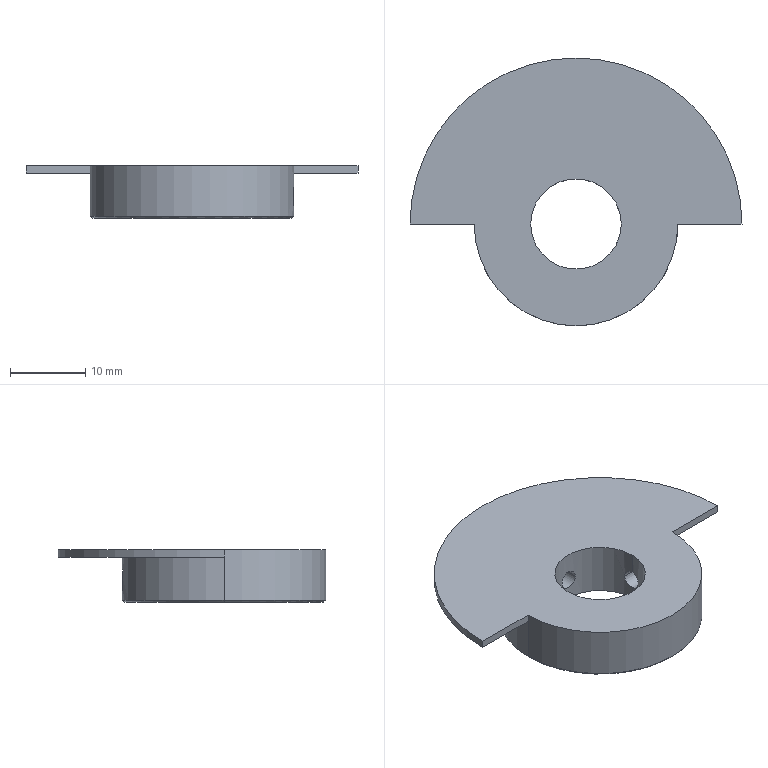Part | NX | 1 solid | 20 faces | box 44 x 35.5 x 7 mm | volume 3612 mm3 | cylinder 9 | plane 5 | spline 4 | cone 2 | commonest cylinder face diameters 2.5 x4 12 x2 27 x2 44 x1
STEP:
#1=CARTESIAN_POINT('',(-13.2,0.,-7.));
#2=VERTEX_POINT('',#1);
#3=CARTESIAN_POINT('',(13.2,0.,-7.));
#4=VERTEX_POINT('',#3);
#5=CARTESIAN_POINT('',(0.,0.,-7.));
#6=DIRECTION('',(0.,0.,-1.));
#7=DIRECTION('',(1.,0.,0.));
#8=AXIS2_PLACEMENT_3D('',#5,#6,#7);
#9=CIRCLE('',#8,13.2);
#10=EDGE_CURVE('',#2,#4,#9,.T.);
#11=ORIENTED_EDGE('',*,*,#10,.T.);
#12=CARTESIAN_POINT('',(0.,0.,-7.));
#13=DIRECTION('',(0.,0.,-1.));
#14=DIRECTION('',(1.,0.,0.));
#15=AXIS2_PLACEMENT_3D('',#12,#13,#14);
#16=CIRCLE('',#15,13.2);
#17=EDGE_CURVE('',#4,#2,#16,.T.);
#18=ORIENTED_EDGE('',*,*,#17,.T.);
#19=EDGE_LOOP('',(#11,#18));
#20=FACE_BOUND('',#19,.T.);
#21=CARTESIAN_POINT('',(-6.,0.,-7.));
#22=VERTEX_POINT('',#21);
#23=CARTESIAN_POINT('',(6.,0.,-7.));
#24=VERTEX_POINT('',#23);
#25=CARTESIAN_POINT('',(0.,0.,-7.));
#26=DIRECTION('',(0.,0.,1.));
#27=DIRECTION('',(1.,0.,0.));
#28=AXIS2_PLACEMENT_3D('',#25,#26,#27);
#29=CIRCLE('',#28,6.);
#30=EDGE_CURVE('',#22,#24,#29,.T.);
#31=ORIENTED_EDGE('',*,*,#30,.T.);
#32=CARTESIAN_POINT('',(0.,0.,-7.));
#33=DIRECTION('',(0.,0.,1.));
#34=DIRECTION('',(1.,0.,0.));
#35=AXIS2_PLACEMENT_3D('',#32,#33,#34);
#36=CIRCLE('',#35,6.);
#37=EDGE_CURVE('',#24,#22,#36,.T.);
#38=ORIENTED_EDGE('',*,*,#37,.T.);
#39=EDGE_LOOP('',(#31,#38));
#40=FACE_BOUND('',#39,.T.);
#41=CARTESIAN_POINT('',(0.,0.,-7.));
#42=DIRECTION('',(0.,0.,1.));
#43=DIRECTION('',(1.,0.,0.));
#44=AXIS2_PLACEMENT_3D('',#41,#42,#43);
#45=PLANE('',#44);
#46=ADVANCED_FACE('',(#20,#40),#45,.F.);
#47=CARTESIAN_POINT('',(-13.5,0.,0.));
#48=VERTEX_POINT('',#47);
#49=CARTESIAN_POINT('',(13.5,0.,0.));
#50=VERTEX_POINT('',#49);
#51=CARTESIAN_POINT('',(0.,0.,0.));
#52=DIRECTION('',(0.,0.,1.));
#53=DIRECTION('',(-1.,0.,0.));
#54=AXIS2_PLACEMENT_3D('',#51,#52,#53);
#55=CIRCLE('',#54,13.5);
#56=EDGE_CURVE('',#48,#50,#55,.T.);
#57=ORIENTED_EDGE('',*,*,#56,.F.);
#58=CARTESIAN_POINT('',(-13.5,0.,-1.));
#59=VERTEX_POINT('',#58);
#60=CARTESIAN_POINT('',(-13.5,0.,0.));
#61=DIRECTION('',(0.,0.,-1.));
#62=VECTOR('',#61,1000.);
#63=LINE('',#60,#62);
#64=EDGE_CURVE('',#48,#59,#63,.T.);
#65=ORIENTED_EDGE('',*,*,#64,.T.);
#66=CARTESIAN_POINT('',(-13.5,0.,-6.7));
#67=VERTEX_POINT('',#66);
#68=CARTESIAN_POINT('',(-13.5,0.,0.));
#69=DIRECTION('',(0.,0.,-1.));
#70=VECTOR('',#69,1000.);
#71=LINE('',#68,#70);
#72=EDGE_CURVE('',#67,#59,#71,.F.);
#73=ORIENTED_EDGE('',*,*,#72,.F.);
#74=CARTESIAN_POINT('',(13.5,0.,-6.7));
#75=VERTEX_POINT('',#74);
#76=CARTESIAN_POINT('',(0.,0.,-6.7));
#77=DIRECTION('',(0.,0.,-1.));
#78=DIRECTION('',(1.,0.,0.));
#79=AXIS2_PLACEMENT_3D('',#76,#77,#78);
#80=CIRCLE('',#79,13.5);
#81=EDGE_CURVE('',#75,#67,#80,.T.);
#82=ORIENTED_EDGE('',*,*,#81,.F.);
#83=CARTESIAN_POINT('',(13.5,0.,-5.7));
#84=VERTEX_POINT('',#83);
#85=CARTESIAN_POINT('',(13.5,0.,0.));
#86=DIRECTION('',(0.,0.,-1.));
#87=VECTOR('',#86,1000.);
#88=LINE('',#85,#87);
#89=EDGE_CURVE('',#84,#75,#88,.T.);
#90=ORIENTED_EDGE('',*,*,#89,.F.);
#91=CARTESIAN_POINT('',(13.5,-0.01096,-5.7));
#92=VERTEX_POINT('',#91);
#93=CARTESIAN_POINT('',(13.5,0.,-5.7));
#94=CARTESIAN_POINT('',(13.5,-0.003653,-5.7));
#95=CARTESIAN_POINT('',(13.5,-0.007306,-5.7));
#96=CARTESIAN_POINT('',(13.5,-0.01096,-5.7));
#97=B_SPLINE_CURVE_WITH_KNOTS('',3,(#93,#94,#95,#96),.UNSPECIFIED.,.F.,.F.,(4,4),(0.,1.),.UNSPECIFIED.);
#98=EDGE_CURVE('',#84,#92,#97,.T.);
#99=ORIENTED_EDGE('',*,*,#98,.T.);
#100=CARTESIAN_POINT('',(13.5,0.,-2.3));
#101=VERTEX_POINT('',#100);
#102=CARTESIAN_POINT('',(13.5,-0.01096,-5.7));
#103=CARTESIAN_POINT('',(13.499,-0.9006,-5.694));
#104=CARTESIAN_POINT('',(13.303,-2.364,-3.994));
#105=CARTESIAN_POINT('',(13.5,-0.8891,-2.3));
#106=CARTESIAN_POINT('',(13.5,0.,-2.3));
#107=B_SPLINE_CURVE_WITH_KNOTS('',3,(#102,#103,#104,#105,#106),.UNSPECIFIED.,.F.,.F.,(4,1,4),(0.,0.5,1.),.UNSPECIFIED.);
#108=EDGE_CURVE('',#92,#101,#107,.T.);
#109=ORIENTED_EDGE('',*,*,#108,.T.);
#110=CARTESIAN_POINT('',(13.5,0.,-1.));
#111=VERTEX_POINT('',#110);
#112=CARTESIAN_POINT('',(13.5,0.,0.));
#113=DIRECTION('',(0.,0.,-1.));
#114=VECTOR('',#113,1000.);
#115=LINE('',#112,#114);
#116=EDGE_CURVE('',#101,#111,#115,.F.);
#117=ORIENTED_EDGE('',*,*,#116,.T.);
#118=CARTESIAN_POINT('',(13.5,0.,0.));
#119=DIRECTION('',(0.,0.,-1.));
#120=VECTOR('',#119,1000.);
#121=LINE('',#118,#120);
#122=EDGE_CURVE('',#50,#111,#121,.T.);
#123=ORIENTED_EDGE('',*,*,#122,.F.);
#124=EDGE_LOOP('',(#57,#65,#73,#82,#90,#99,#109,#117,#123));
#125=FACE_BOUND('',#124,.T.);
#126=CARTESIAN_POINT('',(0.,0.,0.));
#127=DIRECTION('',(0.,0.,-1.));
#128=DIRECTION('',(-1.,0.,0.));
#129=AXIS2_PLACEMENT_3D('',#126,#127,#128);
#130=CYLINDRICAL_SURFACE('',#129,13.5);
#131=ADVANCED_FACE('',(#125),#130,.T.);
#132=CARTESIAN_POINT('',(0.009525,13.24,-5.25));
#133=VERTEX_POINT('',#132);
#134=CARTESIAN_POINT('',(1.25,13.182,-4.));
#135=VERTEX_POINT('',#134);
#136=CARTESIAN_POINT('',(1.25,13.182,-4.));
#137=CARTESIAN_POINT('',(1.25,13.182,-4.158));
#138=CARTESIAN_POINT('',(1.181,13.188,-4.446));
#139=CARTESIAN_POINT('',(1.074,13.198,-4.653));
#140=CARTESIAN_POINT('',(0.8909,13.211,-4.899));
#141=CARTESIAN_POINT('',(0.6426,13.225,-5.08));
#142=CARTESIAN_POINT('',(0.4451,13.234,-5.18));
#143=CARTESIAN_POINT('',(0.1615,13.24,-5.249));
#144=CARTESIAN_POINT('',(0.009525,13.24,-5.25));
#145=B_SPLINE_CURVE_WITH_KNOTS('',3,(#136,#137,#138,#139,#140,#141,#142,#143,#144),.UNSPECIFIED.,.F.,.F.,(4,1,1,1,1,1,4),(0.,0.25,0.375,0.5,0.625,0.75,1.),.UNSPECIFIED.);
#146=EDGE_CURVE('',#133,#135,#145,.F.);
#147=ORIENTED_EDGE('',*,*,#146,.T.);
#148=CARTESIAN_POINT('',(-0.009148,13.24,-2.75));
#149=VERTEX_POINT('',#148);
#150=CARTESIAN_POINT('',(-0.009147,13.24,-2.75));
#151=CARTESIAN_POINT('',(0.1457,13.24,-2.749));
#152=CARTESIAN_POINT('',(0.4278,13.234,-2.813));
#153=CARTESIAN_POINT('',(0.6331,13.225,-2.915));
#154=CARTESIAN_POINT('',(0.8826,13.212,-3.093));
#155=CARTESIAN_POINT('',(1.072,13.198,-3.344));
#156=CARTESIAN_POINT('',(1.178,13.189,-3.548));
#157=CARTESIAN_POINT('',(1.25,13.182,-3.841));
#158=CARTESIAN_POINT('',(1.25,13.182,-4.));
#159=B_SPLINE_CURVE_WITH_KNOTS('',3,(#150,#151,#152,#153,#154,#155,#156,#157,#158),.UNSPECIFIED.,.F.,.F.,(4,1,1,1,1,1,4),(0.,0.25,0.375,0.5,0.625,0.75,1.),.UNSPECIFIED.);
#160=EDGE_CURVE('',#135,#149,#159,.F.);
#161=ORIENTED_EDGE('',*,*,#160,.T.);
#162=CARTESIAN_POINT('',(-0.01305,13.5,-2.3));
#163=VERTEX_POINT('',#162);
#164=CARTESIAN_POINT('',(-0.009148,13.24,-2.75));
#165=CARTESIAN_POINT('',(-0.01305,13.5,-2.3));
#166=B_SPLINE_CURVE_WITH_KNOTS('',1,(#164,#165),.UNSPECIFIED.,.F.,.F.,(2,2),(0.,1.),.UNSPECIFIED.);
#167=EDGE_CURVE('',#163,#149,#166,.F.);
#168=ORIENTED_EDGE('',*,*,#167,.F.);
#169=CARTESIAN_POINT('',(0.01314,13.5,-5.7));
#170=VERTEX_POINT('',#169);
#171=CARTESIAN_POINT('',(0.01314,13.5,-5.7));
#172=CARTESIAN_POINT('',(0.9097,13.499,-5.692));
#173=CARTESIAN_POINT('',(2.362,13.303,-3.98));
#174=CARTESIAN_POINT('',(0.8851,13.501,-2.294));
#175=CARTESIAN_POINT('',(-0.01305,13.5,-2.3));
#176=B_SPLINE_CURVE_WITH_KNOTS('',3,(#171,#172,#173,#174,#175),.UNSPECIFIED.,.F.,.F.,(4,1,4),(0.,0.5,1.),.UNSPECIFIED.);
#177=EDGE_CURVE('',#170,#163,#176,.T.);
#178=ORIENTED_EDGE('',*,*,#177,.F.);
#179=CARTESIAN_POINT('',(0.009525,13.24,-5.25));
#180=CARTESIAN_POINT('',(0.01314,13.5,-5.7));
#181=B_SPLINE_CURVE_WITH_KNOTS('',1,(#179,#180),.UNSPECIFIED.,.F.,.F.,(2,2),(0.,1.),.UNSPECIFIED.);
#182=EDGE_CURVE('',#170,#133,#181,.F.);
#183=ORIENTED_EDGE('',*,*,#182,.T.);
#184=EDGE_LOOP('',(#147,#161,#168,#178,#183));
#185=FACE_BOUND('',#184,.T.);
#186=CARTESIAN_POINT('',(0.009525,13.24,-5.25));
#187=CARTESIAN_POINT('',(0.01314,13.5,-5.7));
#188=CARTESIAN_POINT('',(0.01524,13.24,-5.25));
#189=CARTESIAN_POINT('',(0.02103,13.5,-5.7));
#190=CARTESIAN_POINT('',(0.02096,13.24,-5.25));
#191=CARTESIAN_POINT('',(0.02892,13.5,-5.7));
#192=CARTESIAN_POINT('',(0.05049,13.24,-5.249));
#193=CARTESIAN_POINT('',(0.06965,13.5,-5.699));
#194=CARTESIAN_POINT('',(0.07427,13.24,-5.248));
#195=CARTESIAN_POINT('',(0.1025,13.5,-5.697));
#196=CARTESIAN_POINT('',(0.1973,13.239,-5.238));
#197=CARTESIAN_POINT('',(0.2718,13.498,-5.682));
#198=CARTESIAN_POINT('',(0.295,13.237,-5.219));
#199=CARTESIAN_POINT('',(0.4066,13.494,-5.652));
#200=CARTESIAN_POINT('',(0.586,13.229,-5.123));
#201=CARTESIAN_POINT('',(0.7985,13.479,-5.509));
#202=CARTESIAN_POINT('',(0.7633,13.219,-5.012));
#203=CARTESIAN_POINT('',(1.031,13.462,-5.344));
#204=CARTESIAN_POINT('',(1.05,13.2,-4.71));
#205=CARTESIAN_POINT('',(1.391,13.429,-4.925));
#206=CARTESIAN_POINT('',(1.154,13.191,-4.524));
#207=CARTESIAN_POINT('',(1.516,13.415,-4.679));
#208=CARTESIAN_POINT('',(1.262,13.181,-4.118));
#209=CARTESIAN_POINT('',(1.644,13.4,-4.15));
#210=CARTESIAN_POINT('',(1.264,13.181,-3.902));
#211=CARTESIAN_POINT('',(1.646,13.399,-3.876));
#212=CARTESIAN_POINT('',(1.162,13.19,-3.492));
#213=CARTESIAN_POINT('',(1.525,13.414,-3.342));
#214=CARTESIAN_POINT('',(1.058,13.199,-3.303));
#215=CARTESIAN_POINT('',(1.402,13.428,-3.092));
#216=CARTESIAN_POINT('',(0.7739,13.218,-2.996));
#217=CARTESIAN_POINT('',(1.044,13.461,-2.668));
#218=CARTESIAN_POINT('',(0.5977,13.228,-2.883));
#219=CARTESIAN_POINT('',(0.8144,13.478,-2.501));
#220=CARTESIAN_POINT('',(0.269,13.238,-2.771));
#221=CARTESIAN_POINT('',(0.3717,13.496,-2.333));
#222=CARTESIAN_POINT('',(0.1303,13.24,-2.749));
#223=CARTESIAN_POINT('',(0.1794,13.5,-2.299));
#224=CARTESIAN_POINT('',(-0.009148,13.24,-2.75));
#225=CARTESIAN_POINT('',(-0.01305,13.5,-2.3));
#226=B_SPLINE_SURFACE_WITH_KNOTS('',3,1,((#186,#187),(#188,#189),(#190,#191),(#192,#193),(#194,#195),(#196,#197),(#198,#199),(#200,#201),(#202,#203),(#204,#205),(#206,#207),(#208,#209),(#210,#211),(#212,#213),(#214,#215),(#216,#217),(#218,#219),(#220,#221),(#222,#223),(#224,#225)),.RULED_SURF.,.F.,.F.,.F.,(4,2,2,2,2,2,2,2,2,4),(2,2),(0.,0.02041,0.1054,0.4606,1.192,1.919,2.647,3.381,4.112,4.613),(0.,1.),.UNSPECIFIED.);
#227=ADVANCED_FACE('',(#185),#226,.T.);
#228=CARTESIAN_POINT('',(-22.,0.,-1.));
#229=VERTEX_POINT('',#228);
#230=CARTESIAN_POINT('',(-13.5,0.,-1.));
#231=DIRECTION('',(-1.,0.,0.));
#232=VECTOR('',#231,1000.);
#233=LINE('',#230,#232);
#234=EDGE_CURVE('',#59,#229,#233,.T.);
#235=ORIENTED_EDGE('',*,*,#234,.T.);
#236=CARTESIAN_POINT('',(22.,0.,-1.));
#237=VERTEX_POINT('',#236);
#238=CARTESIAN_POINT('',(0.,0.,-1.));
#239=DIRECTION('',(0.,0.,-1.));
#240=DIRECTION('',(-1.,0.,0.));
#241=AXIS2_PLACEMENT_3D('',#238,#239,#240);
#242=CIRCLE('',#241,22.);
#243=EDGE_CURVE('',#229,#237,#242,.T.);
#244=ORIENTED_EDGE('',*,*,#243,.T.);
#245=CARTESIAN_POINT('',(22.,0.,-1.));
#246=DIRECTION('',(-1.,0.,0.));
#247=VECTOR('',#246,1000.);
#248=LINE('',#245,#247);
#249=EDGE_CURVE('',#237,#111,#248,.T.);
#250=ORIENTED_EDGE('',*,*,#249,.T.);
#251=CARTESIAN_POINT('',(0.,0.,-1.));
#252=DIRECTION('',(0.,0.,1.));
#253=DIRECTION('',(-1.,0.,0.));
#254=AXIS2_PLACEMENT_3D('',#251,#252,#253);
#255=CIRCLE('',#254,13.5);
#256=EDGE_CURVE('',#111,#59,#255,.T.);
#257=ORIENTED_EDGE('',*,*,#256,.T.);
#258=EDGE_LOOP('',(#235,#244,#250,#257));
#259=FACE_BOUND('',#258,.T.);
#260=CARTESIAN_POINT('',(0.,0.,-1.));
#261=DIRECTION('',(0.,0.,1.));
#262=DIRECTION('',(1.,0.,0.));
#263=AXIS2_PLACEMENT_3D('',#260,#261,#262);
#264=PLANE('',#263);
#265=ADVANCED_FACE('',(#259),#264,.F.);
#266=CARTESIAN_POINT('',(-22.,0.,0.));
#267=VERTEX_POINT('',#266);
#268=CARTESIAN_POINT('',(0.,0.,0.));
#269=DIRECTION('',(-1.,0.,0.));
#270=VECTOR('',#269,1000.);
#271=LINE('',#268,#270);
#272=EDGE_CURVE('',#48,#267,#271,.T.);
#273=ORIENTED_EDGE('',*,*,#272,.T.);
#274=CARTESIAN_POINT('',(-22.,0.,0.));
#275=DIRECTION('',(0.,0.,-1.));
#276=VECTOR('',#275,1000.);
#277=LINE('',#274,#276);
#278=EDGE_CURVE('',#267,#229,#277,.T.);
#279=ORIENTED_EDGE('',*,*,#278,.T.);
#280=ORIENTED_EDGE('',*,*,#234,.F.);
#281=ORIENTED_EDGE('',*,*,#64,.F.);
#282=EDGE_LOOP('',(#273,#279,#280,#281));
#283=FACE_BOUND('',#282,.T.);
#284=CARTESIAN_POINT('',(-22.,0.,0.));
#285=DIRECTION('',(0.,1.,0.));
#286=DIRECTION('',(1.,0.,0.));
#287=AXIS2_PLACEMENT_3D('',#284,#285,#286);
#288=PLANE('',#287);
#289=ADVANCED_FACE('',(#283),#288,.F.);
#290=CARTESIAN_POINT('',(22.,0.,0.));
#291=VERTEX_POINT('',#290);
#292=CARTESIAN_POINT('',(0.,0.,0.));
#293=DIRECTION('',(-1.,0.,0.));
#294=VECTOR('',#293,1000.);
#295=LINE('',#292,#294);
#296=EDGE_CURVE('',#291,#50,#295,.T.);
#297=ORIENTED_EDGE('',*,*,#296,.F.);
#298=CARTESIAN_POINT('',(0.,0.,0.));
#299=DIRECTION('',(0.,0.,1.));
#300=DIRECTION('',(-1.,0.,0.));
#301=AXIS2_PLACEMENT_3D('',#298,#299,#300);
#302=CIRCLE('',#301,22.);
#303=EDGE_CURVE('',#291,#267,#302,.T.);
#304=ORIENTED_EDGE('',*,*,#303,.T.);
#305=ORIENTED_EDGE('',*,*,#272,.F.);
#306=ORIENTED_EDGE('',*,*,#56,.T.);
#307=EDGE_LOOP('',(#297,#304,#305,#306));
#308=FACE_BOUND('',#307,.T.);
#309=CARTESIAN_POINT('',(-6.,0.,0.));
#310=VERTEX_POINT('',#309);
#311=CARTESIAN_POINT('',(6.,0.,0.));
#312=VERTEX_POINT('',#311);
#313=CARTESIAN_POINT('',(0.,0.,0.));
#314=DIRECTION('',(0.,0.,1.));
#315=DIRECTION('',(1.,0.,0.));
#316=AXIS2_PLACEMENT_3D('',#313,#314,#315);
#317=CIRCLE('',#316,6.);
#318=EDGE_CURVE('',#310,#312,#317,.T.);
#319=ORIENTED_EDGE('',*,*,#318,.F.);
#320=CARTESIAN_POINT('',(0.,0.,0.));
#321=DIRECTION('',(0.,0.,1.));
#322=DIRECTION('',(1.,0.,0.));
#323=AXIS2_PLACEMENT_3D('',#320,#321,#322);
#324=CIRCLE('',#323,6.);
#325=EDGE_CURVE('',#312,#310,#324,.T.);
#326=ORIENTED_EDGE('',*,*,#325,.F.);
#327=EDGE_LOOP('',(#319,#326));
#328=FACE_BOUND('',#327,.T.);
#329=CARTESIAN_POINT('',(0.,0.,0.));
#330=DIRECTION('',(0.,0.,1.));
#331=DIRECTION('',(1.,0.,0.));
#332=AXIS2_PLACEMENT_3D('',#329,#330,#331);
#333=PLANE('',#332);
#334=ADVANCED_FACE('',(#308,#328),#333,.T.);
#335=ORIENTED_EDGE('',*,*,#318,.T.);
#336=CARTESIAN_POINT('',(6.,0.,-2.75));
#337=VERTEX_POINT('',#336);
#338=CARTESIAN_POINT('',(6.,0.,0.));
#339=DIRECTION('',(0.,0.,-1.));
#340=VECTOR('',#339,1000.);
#341=LINE('',#338,#340);
#342=EDGE_CURVE('',#312,#337,#341,.T.);
#343=ORIENTED_EDGE('',*,*,#342,.T.);
#344=CARTESIAN_POINT('',(5.868,-1.25,-4.));
#345=VERTEX_POINT('',#344);
#346=CARTESIAN_POINT('',(6.,0.,-2.75));
#347=CARTESIAN_POINT('',(6.,-0.6636,-2.75));
#348=CARTESIAN_POINT('',(5.868,-1.25,-3.336));
#349=CARTESIAN_POINT('',(5.868,-1.25,-4.));
#350=B_SPLINE_CURVE_WITH_KNOTS('',3,(#346,#347,#348,#349),.UNSPECIFIED.,.F.,.F.,(4,4),(0.,1.),.UNSPECIFIED.);
#351=EDGE_CURVE('',#345,#337,#350,.F.);
#352=ORIENTED_EDGE('',*,*,#351,.F.);
#353=CARTESIAN_POINT('',(6.,0.,-5.25));
#354=VERTEX_POINT('',#353);
#355=CARTESIAN_POINT('',(5.868,-1.25,-4.));
#356=CARTESIAN_POINT('',(5.868,-1.25,-4.664));
#357=CARTESIAN_POINT('',(6.,-0.6637,-5.25));
#358=CARTESIAN_POINT('',(6.,0.,-5.25));
#359=B_SPLINE_CURVE_WITH_KNOTS('',3,(#355,#356,#357,#358),.UNSPECIFIED.,.F.,.F.,(4,4),(0.,1.),.UNSPECIFIED.);
#360=EDGE_CURVE('',#354,#345,#359,.F.);
#361=ORIENTED_EDGE('',*,*,#360,.F.);
#362=CARTESIAN_POINT('',(6.,0.,0.));
#363=DIRECTION('',(0.,0.,-1.));
#364=VECTOR('',#363,1000.);
#365=LINE('',#362,#364);
#366=EDGE_CURVE('',#24,#354,#365,.F.);
#367=ORIENTED_EDGE('',*,*,#366,.F.);
#368=ORIENTED_EDGE('',*,*,#30,.F.);
#369=CARTESIAN_POINT('',(-6.,0.,0.));
#370=DIRECTION('',(0.,0.,-1.));
#371=VECTOR('',#370,1000.);
#372=LINE('',#369,#371);
#373=EDGE_CURVE('',#22,#310,#372,.F.);
#374=ORIENTED_EDGE('',*,*,#373,.T.);
#375=EDGE_LOOP('',(#335,#343,#352,#361,#367,#368,#374));
#376=FACE_BOUND('',#375,.T.);
#377=CARTESIAN_POINT('',(0.,0.,0.));
#378=DIRECTION('',(0.,0.,-1.));
#379=DIRECTION('',(1.,0.,0.));
#380=AXIS2_PLACEMENT_3D('',#377,#378,#379);
#381=CYLINDRICAL_SURFACE('',#380,6.);
#382=ADVANCED_FACE('',(#376),#381,.F.);
#383=ORIENTED_EDGE('',*,*,#249,.F.);
#384=CARTESIAN_POINT('',(22.,0.,0.));
#385=DIRECTION('',(0.,0.,-1.));
#386=VECTOR('',#385,1000.);
#387=LINE('',#384,#386);
#388=EDGE_CURVE('',#291,#237,#387,.T.);
#389=ORIENTED_EDGE('',*,*,#388,.F.);
#390=ORIENTED_EDGE('',*,*,#296,.T.);
#391=ORIENTED_EDGE('',*,*,#122,.T.);
#392=EDGE_LOOP('',(#383,#389,#390,#391));
#393=FACE_BOUND('',#392,.T.);
#394=CARTESIAN_POINT('',(13.5,0.,0.));
#395=DIRECTION('',(0.,1.,0.));
#396=DIRECTION('',(1.,0.,0.));
#397=AXIS2_PLACEMENT_3D('',#394,#395,#396);
#398=PLANE('',#397);
#399=ADVANCED_FACE('',(#393),#398,.F.);
#400=ORIENTED_EDGE('',*,*,#388,.T.);
#401=ORIENTED_EDGE('',*,*,#243,.F.);
#402=ORIENTED_EDGE('',*,*,#278,.F.);
#403=ORIENTED_EDGE('',*,*,#303,.F.);
#404=EDGE_LOOP('',(#400,#401,#402,#403));
#405=FACE_BOUND('',#404,.T.);
#406=CARTESIAN_POINT('',(0.,0.,0.));
#407=DIRECTION('',(0.,0.,-1.));
#408=DIRECTION('',(-1.,0.,0.));
#409=AXIS2_PLACEMENT_3D('',#406,#407,#408);
#410=CYLINDRICAL_SURFACE('',#409,22.);
#411=ADVANCED_FACE('',(#405),#410,.T.);
#412=CARTESIAN_POINT('',(1.25,5.868,-4.));
#413=VERTEX_POINT('',#412);
#414=CARTESIAN_POINT('',(-1.25,5.868,-4.));
#415=VERTEX_POINT('',#414);
#416=CARTESIAN_POINT('',(1.25,5.868,-4.));
#417=CARTESIAN_POINT('',(1.25,5.868,-3.846));
#418=CARTESIAN_POINT('',(1.18,5.883,-3.553));
#419=CARTESIAN_POINT('',(1.081,5.903,-3.358));
#420=CARTESIAN_POINT('',(0.8926,5.935,-3.103));
#421=CARTESIAN_POINT('',(0.6524,5.965,-2.926));
#422=CARTESIAN_POINT('',(0.4341,5.986,-2.815));
#423=CARTESIAN_POINT('',(0.0001104,6.009,-2.706));
#424=CARTESIAN_POINT('',(-0.4344,5.986,-2.816));
#425=CARTESIAN_POINT('',(-0.6525,5.965,-2.926));
#426=CARTESIAN_POINT('',(-0.8928,5.935,-3.103));
#427=CARTESIAN_POINT('',(-1.081,5.903,-3.359));
#428=CARTESIAN_POINT('',(-1.18,5.883,-3.554));
#429=CARTESIAN_POINT('',(-1.25,5.868,-3.846));
#430=CARTESIAN_POINT('',(-1.25,5.868,-4.));
#431=B_SPLINE_CURVE_WITH_KNOTS('',3,(#416,#417,#418,#419,#420,#421,#422,#423,#424,#425,#426,#427,#428,#429,#430),.UNSPECIFIED.,.F.,.F.,(4,1,1,1,1,1,1,1,1,1,1,1,4),(0.,0.125,0.1875,0.25,0.3125,0.375,0.5,0.625,0.6875,0.75,0.8125,0.875,1.),.UNSPECIFIED.);
#432=EDGE_CURVE('',#413,#415,#431,.T.);
#433=ORIENTED_EDGE('',*,*,#432,.T.);
#434=CARTESIAN_POINT('',(-1.25,13.182,-4.));
#435=VERTEX_POINT('',#434);
#436=CARTESIAN_POINT('',(-1.25,13.5,-4.));
#437=DIRECTION('',(0.,1.,0.));
#438=VECTOR('',#437,1000.);
#439=LINE('',#436,#438);
#440=EDGE_CURVE('',#435,#415,#439,.F.);
#441=ORIENTED_EDGE('',*,*,#440,.F.);
#442=CARTESIAN_POINT('',(-1.25,13.182,-4.));
#443=CARTESIAN_POINT('',(-1.25,13.182,-3.842));
#444=CARTESIAN_POINT('',(-1.179,13.188,-3.551));
#445=CARTESIAN_POINT('',(-1.076,13.197,-3.351));
#446=CARTESIAN_POINT('',(-0.89,13.211,-3.1));
#447=CARTESIAN_POINT('',(-0.6429,13.225,-2.921));
#448=CARTESIAN_POINT('',(-0.4429,13.234,-2.818));
#449=CARTESIAN_POINT('',(-0.1597,13.24,-2.751));
#450=CARTESIAN_POINT('',(-0.009147,13.24,-2.75));
#451=B_SPLINE_CURVE_WITH_KNOTS('',3,(#442,#443,#444,#445,#446,#447,#448,#449,#450),.UNSPECIFIED.,.F.,.F.,(4,1,1,1,1,1,4),(0.,0.25,0.375,0.5,0.625,0.75,1.),.UNSPECIFIED.);
#452=EDGE_CURVE('',#149,#435,#451,.F.);
#453=ORIENTED_EDGE('',*,*,#452,.F.);
#454=ORIENTED_EDGE('',*,*,#160,.F.);
#455=CARTESIAN_POINT('',(1.25,13.5,-4.));
#456=DIRECTION('',(0.,1.,0.));
#457=VECTOR('',#456,1000.);
#458=LINE('',#455,#457);
#459=EDGE_CURVE('',#135,#413,#458,.F.);
#460=ORIENTED_EDGE('',*,*,#459,.T.);
#461=EDGE_LOOP('',(#433,#441,#453,#454,#460));
#462=FACE_BOUND('',#461,.T.);
#463=CARTESIAN_POINT('',(0.,13.5,-4.));
#464=DIRECTION('',(0.,1.,0.));
#465=DIRECTION('',(1.,0.,0.));
#466=AXIS2_PLACEMENT_3D('',#463,#464,#465);
#467=CYLINDRICAL_SURFACE('',#466,1.25);
#468=ADVANCED_FACE('',(#462),#467,.F.);
#469=CARTESIAN_POINT('',(5.868,1.25,-4.));
#470=VERTEX_POINT('',#469);
#471=CARTESIAN_POINT('',(6.,0.,-2.75));
#472=CARTESIAN_POINT('',(6.,0.1552,-2.75));
#473=CARTESIAN_POINT('',(5.986,0.4429,-2.818));
#474=CARTESIAN_POINT('',(5.966,0.6476,-2.923));
#475=CARTESIAN_POINT('',(5.935,0.8941,-3.104));
#476=CARTESIAN_POINT('',(5.903,1.079,-3.357));
#477=CARTESIAN_POINT('',(5.883,1.181,-3.555));
#478=CARTESIAN_POINT('',(5.868,1.25,-3.845));
#479=CARTESIAN_POINT('',(5.868,1.25,-4.));
#480=B_SPLINE_CURVE_WITH_KNOTS('',3,(#471,#472,#473,#474,#475,#476,#477,#478,#479),.UNSPECIFIED.,.F.,.F.,(4,1,1,1,1,1,4),(0.,0.25,0.375,0.5,0.625,0.75,1.),.UNSPECIFIED.);
#481=EDGE_CURVE('',#337,#470,#480,.T.);
#482=ORIENTED_EDGE('',*,*,#481,.T.);
#483=CARTESIAN_POINT('',(13.182,1.25,-4.));
#484=VERTEX_POINT('',#483);
#485=CARTESIAN_POINT('',(13.5,1.25,-4.));
#486=DIRECTION('',(1.,0.,0.));
#487=VECTOR('',#486,1000.);
#488=LINE('',#485,#487);
#489=EDGE_CURVE('',#470,#484,#488,.T.);
#490=ORIENTED_EDGE('',*,*,#489,.T.);
#491=CARTESIAN_POINT('',(13.24,0.008007,-2.75));
#492=VERTEX_POINT('',#491);
#493=CARTESIAN_POINT('',(13.182,1.25,-4.));
#494=CARTESIAN_POINT('',(13.182,1.25,-3.842));
#495=CARTESIAN_POINT('',(13.188,1.181,-3.553));
#496=CARTESIAN_POINT('',(13.198,1.074,-3.347));
#497=CARTESIAN_POINT('',(13.211,0.8903,-3.101));
#498=CARTESIAN_POINT('',(13.225,0.642,-2.92));
#499=CARTESIAN_POINT('',(13.234,0.4439,-2.819));
#500=CARTESIAN_POINT('',(13.24,0.1601,-2.751));
#501=CARTESIAN_POINT('',(13.24,0.008007,-2.75));
#502=B_SPLINE_CURVE_WITH_KNOTS('',3,(#493,#494,#495,#496,#497,#498,#499,#500,#501),.UNSPECIFIED.,.F.,.F.,(4,1,1,1,1,1,4),(0.,0.25,0.375,0.5,0.625,0.75,1.),.UNSPECIFIED.);
#503=EDGE_CURVE('',#492,#484,#502,.F.);
#504=ORIENTED_EDGE('',*,*,#503,.F.);
#505=CARTESIAN_POINT('',(13.182,-1.25,-4.));
#506=VERTEX_POINT('',#505);
#507=CARTESIAN_POINT('',(13.24,0.008007,-2.75));
#508=CARTESIAN_POINT('',(13.24,-0.1434,-2.749));
#509=CARTESIAN_POINT('',(13.234,-0.4295,-2.813));
#510=CARTESIAN_POINT('',(13.225,-0.6323,-2.914));
#511=CARTESIAN_POINT('',(13.212,-0.8837,-3.094));
#512=CARTESIAN_POINT('',(13.198,-1.072,-3.345));
#513=CARTESIAN_POINT('',(13.189,-1.179,-3.547));
#514=CARTESIAN_POINT('',(13.182,-1.25,-3.845));
#515=CARTESIAN_POINT('',(13.182,-1.25,-4.));
#516=B_SPLINE_CURVE_WITH_KNOTS('',3,(#507,#508,#509,#510,#511,#512,#513,#514,#515),.UNSPECIFIED.,.F.,.F.,(4,1,1,1,1,1,4),(0.,0.25,0.375,0.5,0.625,0.75,1.),.UNSPECIFIED.);
#517=EDGE_CURVE('',#506,#492,#516,.F.);
#518=ORIENTED_EDGE('',*,*,#517,.F.);
#519=CARTESIAN_POINT('',(13.5,-1.25,-4.));
#520=DIRECTION('',(1.,0.,0.));
#521=VECTOR('',#520,1000.);
#522=LINE('',#519,#521);
#523=EDGE_CURVE('',#345,#506,#522,.T.);
#524=ORIENTED_EDGE('',*,*,#523,.F.);
#525=ORIENTED_EDGE('',*,*,#351,.T.);
#526=EDGE_LOOP('',(#482,#490,#504,#518,#524,#525));
#527=FACE_BOUND('',#526,.T.);
#528=CARTESIAN_POINT('',(13.5,0.,-4.));
#529=DIRECTION('',(1.,0.,0.));
#530=DIRECTION('',(0.,-1.,0.));
#531=AXIS2_PLACEMENT_3D('',#528,#529,#530);
#532=CYLINDRICAL_SURFACE('',#531,1.25);
#533=ADVANCED_FACE('',(#527),#532,.F.);
#534=CARTESIAN_POINT('',(13.5,0.01105,-2.3));
#535=VERTEX_POINT('',#534);
#536=CARTESIAN_POINT('',(13.5,0.01105,-2.3));
#537=CARTESIAN_POINT('',(13.499,0.9058,-2.306));
#538=CARTESIAN_POINT('',(13.303,2.358,-4.01));
#539=CARTESIAN_POINT('',(13.5,0.896,-5.699));
#540=CARTESIAN_POINT('',(13.5,0.,-5.7));
#541=B_SPLINE_CURVE_WITH_KNOTS('',3,(#536,#537,#538,#539,#540),.UNSPECIFIED.,.F.,.F.,(4,1,4),(0.,0.5,1.),.UNSPECIFIED.);
#542=EDGE_CURVE('',#535,#84,#541,.T.);
#543=ORIENTED_EDGE('',*,*,#542,.F.);
#544=CARTESIAN_POINT('',(13.24,0.008007,-2.75));
#545=CARTESIAN_POINT('',(13.5,0.01105,-2.3));
#546=B_SPLINE_CURVE_WITH_KNOTS('',1,(#544,#545),.UNSPECIFIED.,.F.,.F.,(2,2),(0.,1.),.UNSPECIFIED.);
#547=EDGE_CURVE('',#535,#492,#546,.F.);
#548=ORIENTED_EDGE('',*,*,#547,.T.);
#549=ORIENTED_EDGE('',*,*,#503,.T.);
#550=CARTESIAN_POINT('',(13.24,-0.007631,-5.25));
#551=VERTEX_POINT('',#550);
#552=CARTESIAN_POINT('',(13.24,-0.00763,-5.25));
#553=CARTESIAN_POINT('',(13.24,0.1471,-5.251));
#554=CARTESIAN_POINT('',(13.234,0.4291,-5.187));
#555=CARTESIAN_POINT('',(13.225,0.6337,-5.085));
#556=CARTESIAN_POINT('',(13.212,0.8832,-4.907));
#557=CARTESIAN_POINT('',(13.198,1.072,-4.656));
#558=CARTESIAN_POINT('',(13.189,1.179,-4.452));
#559=CARTESIAN_POINT('',(13.182,1.25,-4.159));
#560=CARTESIAN_POINT('',(13.182,1.25,-4.));
#561=B_SPLINE_CURVE_WITH_KNOTS('',3,(#552,#553,#554,#555,#556,#557,#558,#559,#560),.UNSPECIFIED.,.F.,.F.,(4,1,1,1,1,1,4),(0.,0.25,0.375,0.5,0.625,0.75,1.),.UNSPECIFIED.);
#562=EDGE_CURVE('',#484,#551,#561,.F.);
#563=ORIENTED_EDGE('',*,*,#562,.T.);
#564=CARTESIAN_POINT('',(13.24,-0.007631,-5.25));
#565=CARTESIAN_POINT('',(13.5,-0.01096,-5.7));
#566=B_SPLINE_CURVE_WITH_KNOTS('',1,(#564,#565),.UNSPECIFIED.,.F.,.F.,(2,2),(0.,1.),.UNSPECIFIED.);
#567=EDGE_CURVE('',#92,#551,#566,.F.);
#568=ORIENTED_EDGE('',*,*,#567,.F.);
#569=ORIENTED_EDGE('',*,*,#98,.F.);
#570=EDGE_LOOP('',(#543,#548,#549,#563,#568,#569));
#571=FACE_BOUND('',#570,.T.);
#572=CARTESIAN_POINT('',(13.24,0.008007,-2.75));
#573=CARTESIAN_POINT('',(13.5,0.01105,-2.3));
#574=CARTESIAN_POINT('',(13.24,0.01372,-2.75));
#575=CARTESIAN_POINT('',(13.5,0.01893,-2.3));
#576=CARTESIAN_POINT('',(13.24,0.01944,-2.75));
#577=CARTESIAN_POINT('',(13.5,0.02682,-2.3));
#578=CARTESIAN_POINT('',(13.24,0.04897,-2.751));
#579=CARTESIAN_POINT('',(13.5,0.06756,-2.301));
#580=CARTESIAN_POINT('',(13.24,0.07275,-2.752));
#581=CARTESIAN_POINT('',(13.5,0.1004,-2.303));
#582=CARTESIAN_POINT('',(13.239,0.1958,-2.761));
#583=CARTESIAN_POINT('',(13.498,0.2697,-2.318));
#584=CARTESIAN_POINT('',(13.237,0.2935,-2.781));
#585=CARTESIAN_POINT('',(13.495,0.4045,-2.348));
#586=CARTESIAN_POINT('',(13.229,0.5846,-2.876));
#587=CARTESIAN_POINT('',(13.479,0.7967,-2.49));
#588=CARTESIAN_POINT('',(13.219,0.7622,-2.987));
#589=CARTESIAN_POINT('',(13.462,1.029,-2.655));
#590=CARTESIAN_POINT('',(13.2,1.049,-3.289));
#591=CARTESIAN_POINT('',(13.429,1.39,-3.073));
#592=CARTESIAN_POINT('',(13.191,1.154,-3.475));
#593=CARTESIAN_POINT('',(13.415,1.515,-3.319));
#594=CARTESIAN_POINT('',(13.181,1.262,-3.881));
#595=CARTESIAN_POINT('',(13.4,1.644,-3.849));
#596=CARTESIAN_POINT('',(13.181,1.264,-4.097));
#597=CARTESIAN_POINT('',(13.399,1.646,-4.123));
#598=CARTESIAN_POINT('',(13.19,1.162,-4.507));
#599=CARTESIAN_POINT('',(13.414,1.525,-4.657));
#600=CARTESIAN_POINT('',(13.199,1.059,-4.697));
#601=CARTESIAN_POINT('',(13.428,1.402,-4.908));
#602=CARTESIAN_POINT('',(13.218,0.7742,-5.003));
#603=CARTESIAN_POINT('',(13.461,1.045,-5.332));
#604=CARTESIAN_POINT('',(13.228,0.598,-5.117));
#605=CARTESIAN_POINT('',(13.478,0.8148,-5.499));
#606=CARTESIAN_POINT('',(13.238,0.2698,-5.229));
#607=CARTESIAN_POINT('',(13.496,0.3728,-5.667));
#608=CARTESIAN_POINT('',(13.24,0.1314,-5.251));
#609=CARTESIAN_POINT('',(13.5,0.181,-5.701));
#610=CARTESIAN_POINT('',(13.24,-0.007631,-5.25));
#611=CARTESIAN_POINT('',(13.5,-0.01096,-5.7));
#612=CARTESIAN_POINT('',(13.24,-0.01533,-5.25));
#613=CARTESIAN_POINT('',(13.5,-0.02159,-5.7));
#614=CARTESIAN_POINT('',(13.24,-0.02303,-5.25));
#615=CARTESIAN_POINT('',(13.5,-0.03222,-5.7));
#616=CARTESIAN_POINT('',(13.24,-0.03073,-5.25));
#617=CARTESIAN_POINT('',(13.5,-0.04285,-5.7));
#618=B_SPLINE_SURFACE_WITH_KNOTS('',3,1,((#572,#573),(#574,#575),(#576,#577),(#578,#579),(#580,#581),(#582,#583),(#584,#585),(#586,#587),(#588,#589),(#590,#591),(#592,#593),(#594,#595),(#596,#597),(#598,#599),(#600,#601),(#602,#603),(#604,#605),(#606,#607),(#608,#609),(#610,#611),(#612,#613),(#614,#615),(#616,#617)),.RULED_SURF.,.F.,.F.,.F.,(4,2,2,2,2,2,2,2,2,3,4),(2,2),(0.,0.02041,0.1054,0.4605,1.193,1.92,2.648,3.383,4.114,4.613,4.641),(0.,1.),.UNSPECIFIED.);
#619=ADVANCED_FACE('',(#571),#618,.T.);
#620=ORIENTED_EDGE('',*,*,#10,.F.);
#621=CARTESIAN_POINT('',(-13.5,0.,-6.7));
#622=DIRECTION('',(-0.7071,0.,0.7071));
#623=VECTOR('',#622,1000.);
#624=LINE('',#621,#623);
#625=EDGE_CURVE('',#2,#67,#624,.T.);
#626=ORIENTED_EDGE('',*,*,#625,.T.);
#627=CARTESIAN_POINT('',(0.,0.,-6.7));
#628=DIRECTION('',(0.,0.,-1.));
#629=DIRECTION('',(1.,0.,0.));
#630=AXIS2_PLACEMENT_3D('',#627,#628,#629);
#631=CIRCLE('',#630,13.5);
#632=EDGE_CURVE('',#67,#75,#631,.T.);
#633=ORIENTED_EDGE('',*,*,#632,.T.);
#634=CARTESIAN_POINT('',(13.5,0.,-6.7));
#635=DIRECTION('',(0.7071,0.,0.7071));
#636=VECTOR('',#635,1000.);
#637=LINE('',#634,#636);
#638=EDGE_CURVE('',#4,#75,#637,.T.);
#639=ORIENTED_EDGE('',*,*,#638,.F.);
#640=EDGE_LOOP('',(#620,#626,#633,#639));
#641=FACE_BOUND('',#640,.T.);
#642=CARTESIAN_POINT('',(0.,0.,-6.7));
#643=DIRECTION('',(0.,0.,1.));
#644=DIRECTION('',(1.,0.,0.));
#645=AXIS2_PLACEMENT_3D('',#642,#643,#644);
#646=CONICAL_SURFACE('',#645,13.5,0.7854);
#647=ADVANCED_FACE('',(#641),#646,.T.);
#648=ORIENTED_EDGE('',*,*,#146,.F.);
#649=CARTESIAN_POINT('',(0.009525,13.24,-5.25));
#650=CARTESIAN_POINT('',(-0.1421,13.24,-5.251));
#651=CARTESIAN_POINT('',(-0.4283,13.234,-5.187));
#652=CARTESIAN_POINT('',(-0.6317,13.225,-5.086));
#653=CARTESIAN_POINT('',(-0.8831,13.212,-4.907));
#654=CARTESIAN_POINT('',(-1.072,13.198,-4.655));
#655=CARTESIAN_POINT('',(-1.178,13.189,-4.454));
#656=CARTESIAN_POINT('',(-1.25,13.182,-4.155));
#657=CARTESIAN_POINT('',(-1.25,13.182,-4.));
#658=B_SPLINE_CURVE_WITH_KNOTS('',3,(#649,#650,#651,#652,#653,#654,#655,#656,#657),.UNSPECIFIED.,.F.,.F.,(4,1,1,1,1,1,4),(0.,0.25,0.375,0.5,0.625,0.75,1.),.UNSPECIFIED.);
#659=EDGE_CURVE('',#435,#133,#658,.F.);
#660=ORIENTED_EDGE('',*,*,#659,.F.);
#661=ORIENTED_EDGE('',*,*,#440,.T.);
#662=CARTESIAN_POINT('',(-1.25,5.868,-4.));
#663=CARTESIAN_POINT('',(-1.25,5.868,-4.153));
#664=CARTESIAN_POINT('',(-1.18,5.883,-4.447));
#665=CARTESIAN_POINT('',(-1.081,5.903,-4.641));
#666=CARTESIAN_POINT('',(-0.8923,5.935,-4.897));
#667=CARTESIAN_POINT('',(-0.6523,5.965,-5.074));
#668=CARTESIAN_POINT('',(-0.4339,5.986,-5.185));
#669=CARTESIAN_POINT('',(-0.0001315,6.009,-5.294));
#670=CARTESIAN_POINT('',(0.4343,5.986,-5.185));
#671=CARTESIAN_POINT('',(0.6522,5.965,-5.074));
#672=CARTESIAN_POINT('',(0.8923,5.935,-4.897));
#673=CARTESIAN_POINT('',(1.081,5.903,-4.641));
#674=CARTESIAN_POINT('',(1.18,5.883,-4.447));
#675=CARTESIAN_POINT('',(1.25,5.868,-4.153));
#676=CARTESIAN_POINT('',(1.25,5.868,-4.));
#677=B_SPLINE_CURVE_WITH_KNOTS('',3,(#662,#663,#664,#665,#666,#667,#668,#669,#670,#671,#672,#673,#674,#675,#676),.UNSPECIFIED.,.F.,.F.,(4,1,1,1,1,1,1,1,1,1,1,1,4),(0.,0.125,0.1875,0.25,0.3125,0.375,0.5,0.625,0.6875,0.75,0.8125,0.875,1.),.UNSPECIFIED.);
#678=EDGE_CURVE('',#415,#413,#677,.T.);
#679=ORIENTED_EDGE('',*,*,#678,.T.);
#680=ORIENTED_EDGE('',*,*,#459,.F.);
#681=EDGE_LOOP('',(#648,#660,#661,#679,#680));
#682=FACE_BOUND('',#681,.T.);
#683=CARTESIAN_POINT('',(0.,13.5,-4.));
#684=DIRECTION('',(0.,1.,0.));
#685=DIRECTION('',(1.,0.,0.));
#686=AXIS2_PLACEMENT_3D('',#683,#684,#685);
#687=CYLINDRICAL_SURFACE('',#686,1.25);
#688=ADVANCED_FACE('',(#682),#687,.F.);
#689=ORIENTED_EDGE('',*,*,#632,.F.);
#690=ORIENTED_EDGE('',*,*,#72,.T.);
#691=ORIENTED_EDGE('',*,*,#256,.F.);
#692=ORIENTED_EDGE('',*,*,#116,.F.);
#693=CARTESIAN_POINT('',(13.5,0.,-2.3));
#694=CARTESIAN_POINT('',(13.5,0.003678,-2.3));
#695=CARTESIAN_POINT('',(13.5,0.007364,-2.3));
#696=CARTESIAN_POINT('',(13.5,0.01105,-2.3));
#697=B_SPLINE_CURVE_WITH_KNOTS('',3,(#693,#694,#695,#696),.UNSPECIFIED.,.F.,.F.,(4,4),(9.217,9.227),.UNSPECIFIED.);
#698=EDGE_CURVE('',#101,#535,#697,.T.);
#699=ORIENTED_EDGE('',*,*,#698,.T.);
#700=ORIENTED_EDGE('',*,*,#542,.T.);
#701=ORIENTED_EDGE('',*,*,#89,.T.);
#702=EDGE_LOOP('',(#689,#690,#691,#692,#699,#700,#701));
#703=FACE_BOUND('',#702,.T.);
#704=CARTESIAN_POINT('',(-0.01305,13.5,-2.3));
#705=CARTESIAN_POINT('',(-0.4588,13.5,-2.304));
#706=CARTESIAN_POINT('',(-1.317,13.446,-2.721));
#707=CARTESIAN_POINT('',(-1.791,13.378,-4.012));
#708=CARTESIAN_POINT('',(-1.298,13.448,-5.302));
#709=CARTESIAN_POINT('',(-0.4329,13.5,-5.704));
#710=CARTESIAN_POINT('',(0.01314,13.5,-5.7));
#711=B_SPLINE_CURVE_WITH_KNOTS('',3,(#704,#705,#706,#707,#708,#709,#710),.UNSPECIFIED.,.F.,.F.,(4,1,1,1,4),(0.,0.25,0.5,0.75,1.),.UNSPECIFIED.);
#712=EDGE_CURVE('',#163,#170,#711,.T.);
#713=ORIENTED_EDGE('',*,*,#712,.T.);
#714=ORIENTED_EDGE('',*,*,#177,.T.);
#715=EDGE_LOOP('',(#713,#714));
#716=FACE_BOUND('',#715,.T.);
#717=CARTESIAN_POINT('',(0.,0.,0.));
#718=DIRECTION('',(0.,0.,-1.));
#719=DIRECTION('',(-1.,0.,0.));
#720=AXIS2_PLACEMENT_3D('',#717,#718,#719);
#721=CYLINDRICAL_SURFACE('',#720,13.5);
#722=ADVANCED_FACE('',(#703,#716),#721,.T.);
#723=ORIENTED_EDGE('',*,*,#489,.F.);
#724=CARTESIAN_POINT('',(5.868,1.25,-4.));
#725=CARTESIAN_POINT('',(5.868,1.25,-4.155));
#726=CARTESIAN_POINT('',(5.883,1.181,-4.446));
#727=CARTESIAN_POINT('',(5.903,1.079,-4.643));
#728=CARTESIAN_POINT('',(5.935,0.8941,-4.896));
#729=CARTESIAN_POINT('',(5.966,0.6477,-5.076));
#730=CARTESIAN_POINT('',(5.986,0.4428,-5.182));
#731=CARTESIAN_POINT('',(6.,0.1552,-5.25));
#732=CARTESIAN_POINT('',(6.,0.,-5.25));
#733=B_SPLINE_CURVE_WITH_KNOTS('',3,(#724,#725,#726,#727,#728,#729,#730,#731,#732),.UNSPECIFIED.,.F.,.F.,(4,1,1,1,1,1,4),(0.,0.25,0.375,0.5,0.625,0.75,1.),.UNSPECIFIED.);
#734=EDGE_CURVE('',#470,#354,#733,.T.);
#735=ORIENTED_EDGE('',*,*,#734,.T.);
#736=ORIENTED_EDGE('',*,*,#360,.T.);
#737=ORIENTED_EDGE('',*,*,#523,.T.);
#738=CARTESIAN_POINT('',(13.182,-1.25,-4.));
#739=CARTESIAN_POINT('',(13.182,-1.25,-4.158));
#740=CARTESIAN_POINT('',(13.188,-1.179,-4.449));
#741=CARTESIAN_POINT('',(13.197,-1.076,-4.649));
#742=CARTESIAN_POINT('',(13.211,-0.8894,-4.9));
#743=CARTESIAN_POINT('',(13.225,-0.6423,-5.08));
#744=CARTESIAN_POINT('',(13.234,-0.4417,-5.182));
#745=CARTESIAN_POINT('',(13.24,-0.1583,-5.249));
#746=CARTESIAN_POINT('',(13.24,-0.00763,-5.25));
#747=B_SPLINE_CURVE_WITH_KNOTS('',3,(#738,#739,#740,#741,#742,#743,#744,#745,#746),.UNSPECIFIED.,.F.,.F.,(4,1,1,1,1,1,4),(0.,0.25,0.375,0.5,0.625,0.75,1.),.UNSPECIFIED.);
#748=EDGE_CURVE('',#551,#506,#747,.F.);
#749=ORIENTED_EDGE('',*,*,#748,.F.);
#750=ORIENTED_EDGE('',*,*,#562,.F.);
#751=EDGE_LOOP('',(#723,#735,#736,#737,#749,#750));
#752=FACE_BOUND('',#751,.T.);
#753=CARTESIAN_POINT('',(13.5,0.,-4.));
#754=DIRECTION('',(1.,0.,0.));
#755=DIRECTION('',(0.,-1.,0.));
#756=AXIS2_PLACEMENT_3D('',#753,#754,#755);
#757=CYLINDRICAL_SURFACE('',#756,1.25);
#758=ADVANCED_FACE('',(#752),#757,.F.);
#759=ORIENTED_EDGE('',*,*,#638,.T.);
#760=ORIENTED_EDGE('',*,*,#81,.T.);
#761=ORIENTED_EDGE('',*,*,#625,.F.);
#762=ORIENTED_EDGE('',*,*,#17,.F.);
#763=EDGE_LOOP('',(#759,#760,#761,#762));
#764=FACE_BOUND('',#763,.T.);
#765=CARTESIAN_POINT('',(0.,0.,-6.7));
#766=DIRECTION('',(0.,0.,1.));
#767=DIRECTION('',(1.,0.,0.));
#768=AXIS2_PLACEMENT_3D('',#765,#766,#767);
#769=CONICAL_SURFACE('',#768,13.5,0.7854);
#770=ADVANCED_FACE('',(#764),#769,.T.);
#771=ORIENTED_EDGE('',*,*,#481,.F.);
#772=ORIENTED_EDGE('',*,*,#342,.F.);
#773=ORIENTED_EDGE('',*,*,#325,.T.);
#774=ORIENTED_EDGE('',*,*,#373,.F.);
#775=ORIENTED_EDGE('',*,*,#37,.F.);
#776=ORIENTED_EDGE('',*,*,#366,.T.);
#777=ORIENTED_EDGE('',*,*,#734,.F.);
#778=EDGE_LOOP('',(#771,#772,#773,#774,#775,#776,#777));
#779=FACE_BOUND('',#778,.T.);
#780=ORIENTED_EDGE('',*,*,#432,.F.);
#781=ORIENTED_EDGE('',*,*,#678,.F.);
#782=EDGE_LOOP('',(#780,#781));
#783=FACE_BOUND('',#782,.T.);
#784=CARTESIAN_POINT('',(0.,0.,0.));
#785=DIRECTION('',(0.,0.,-1.));
#786=DIRECTION('',(1.,0.,0.));
#787=AXIS2_PLACEMENT_3D('',#784,#785,#786);
#788=CYLINDRICAL_SURFACE('',#787,6.);
#789=ADVANCED_FACE('',(#779,#783),#788,.F.);
#790=ORIENTED_EDGE('',*,*,#167,.T.);
#791=ORIENTED_EDGE('',*,*,#452,.T.);
#792=ORIENTED_EDGE('',*,*,#659,.T.);
#793=ORIENTED_EDGE('',*,*,#182,.F.);
#794=ORIENTED_EDGE('',*,*,#712,.F.);
#795=EDGE_LOOP('',(#790,#791,#792,#793,#794));
#796=FACE_BOUND('',#795,.T.);
#797=CARTESIAN_POINT('',(-0.009148,13.24,-2.75));
#798=CARTESIAN_POINT('',(-0.01305,13.5,-2.3));
#799=CARTESIAN_POINT('',(-0.07196,13.24,-2.75));
#800=CARTESIAN_POINT('',(-0.09975,13.5,-2.301));
#801=CARTESIAN_POINT('',(-0.1349,13.24,-2.756));
#802=CARTESIAN_POINT('',(-0.1865,13.499,-2.309));
#803=CARTESIAN_POINT('',(-0.3998,13.236,-2.798));
#804=CARTESIAN_POINT('',(-0.5485,13.492,-2.373));
#805=CARTESIAN_POINT('',(-0.5907,13.228,-2.879));
#806=CARTESIAN_POINT('',(-0.8061,13.478,-2.497));
#807=CARTESIAN_POINT('',(-0.9215,13.209,-3.13));
#808=CARTESIAN_POINT('',(-1.233,13.445,-2.855));
#809=CARTESIAN_POINT('',(-1.055,13.199,-3.297));
#810=CARTESIAN_POINT('',(-1.396,13.428,-3.083));
#811=CARTESIAN_POINT('',(-1.227,13.185,-3.681));
#812=CARTESIAN_POINT('',(-1.603,13.405,-3.591));
#813=CARTESIAN_POINT('',(-1.263,13.181,-3.894));
#814=CARTESIAN_POINT('',(-1.645,13.399,-3.862));
#815=CARTESIAN_POINT('',(-1.228,13.184,-4.314));
#816=CARTESIAN_POINT('',(-1.604,13.404,-4.406));
#817=CARTESIAN_POINT('',(-1.157,13.191,-4.518));
#818=CARTESIAN_POINT('',(-1.521,13.415,-4.669));
#819=CARTESIAN_POINT('',(-0.925,13.209,-4.866));
#820=CARTESIAN_POINT('',(-1.235,13.444,-5.14));
#821=CARTESIAN_POINT('',(-0.7682,13.219,-5.007));
#822=CARTESIAN_POINT('',(-1.037,13.462,-5.34));
#823=CARTESIAN_POINT('',(-0.4042,13.235,-5.201));
#824=CARTESIAN_POINT('',(-0.5571,13.491,-5.622));
#825=CARTESIAN_POINT('',(-0.2041,13.24,-5.25));
#826=CARTESIAN_POINT('',(-0.2808,13.5,-5.7));
#827=CARTESIAN_POINT('',(0.003196,13.24,-5.25));
#828=CARTESIAN_POINT('',(0.004398,13.5,-5.7));
#829=CARTESIAN_POINT('',(0.006359,13.24,-5.25));
#830=CARTESIAN_POINT('',(0.008773,13.5,-5.7));
#831=CARTESIAN_POINT('',(0.009525,13.24,-5.25));
#832=CARTESIAN_POINT('',(0.01314,13.5,-5.7));
#833=B_SPLINE_SURFACE_WITH_KNOTS('',3,1,((#797,#798),(#799,#800),(#801,#802),(#803,#804),(#805,#806),(#807,#808),(#809,#810),(#811,#812),(#813,#814),(#815,#816),(#817,#818),(#819,#820),(#821,#822),(#823,#824),(#825,#826),(#827,#828),(#829,#830),(#831,#832)),.RULED_SURF.,.F.,.F.,.F.,(4,2,2,2,2,2,2,2,4),(2,2),(4.613,4.839,5.568,6.302,7.029,7.759,8.489,9.216,9.227),(0.,1.),.UNSPECIFIED.);
#834=ADVANCED_FACE('',(#796),#833,.T.);
#835=ORIENTED_EDGE('',*,*,#567,.T.);
#836=ORIENTED_EDGE('',*,*,#748,.T.);
#837=ORIENTED_EDGE('',*,*,#517,.T.);
#838=ORIENTED_EDGE('',*,*,#547,.F.);
#839=ORIENTED_EDGE('',*,*,#698,.F.);
#840=ORIENTED_EDGE('',*,*,#108,.F.);
#841=EDGE_LOOP('',(#835,#836,#837,#838,#839,#840));
#842=FACE_BOUND('',#841,.T.);
#843=CARTESIAN_POINT('',(13.24,0.01547,-5.25));
#844=CARTESIAN_POINT('',(13.327,0.01729,-5.4));
#845=CARTESIAN_POINT('',(13.413,0.01911,-5.55));
#846=CARTESIAN_POINT('',(13.5,0.02093,-5.7));
#847=CARTESIAN_POINT('',(13.24,-0.3073,-5.248));
#848=CARTESIAN_POINT('',(13.327,-0.3464,-5.398));
#849=CARTESIAN_POINT('',(13.413,-0.3855,-5.548));
#850=CARTESIAN_POINT('',(13.5,-0.4246,-5.697));
#851=CARTESIAN_POINT('',(13.227,-0.633,-5.127));
#852=CARTESIAN_POINT('',(13.31,-0.7103,-5.253));
#853=CARTESIAN_POINT('',(13.393,-0.7877,-5.38));
#854=CARTESIAN_POINT('',(13.476,-0.865,-5.506));
#855=CARTESIAN_POINT('',(13.197,-1.106,-4.669));
#856=CARTESIAN_POINT('',(13.272,-1.225,-4.735));
#857=CARTESIAN_POINT('',(13.348,-1.344,-4.802));
#858=CARTESIAN_POINT('',(13.424,-1.463,-4.868));
#859=CARTESIAN_POINT('',(13.182,-1.249,-4.339));
#860=CARTESIAN_POINT('',(13.255,-1.375,-4.372));
#861=CARTESIAN_POINT('',(13.329,-1.502,-4.405));
#862=CARTESIAN_POINT('',(13.402,-1.629,-4.438));
#863=CARTESIAN_POINT('',(13.182,-1.251,-3.669));
#864=CARTESIAN_POINT('',(13.255,-1.378,-3.637));
#865=CARTESIAN_POINT('',(13.328,-1.504,-3.605));
#866=CARTESIAN_POINT('',(13.401,-1.631,-3.574));
#867=CARTESIAN_POINT('',(13.196,-1.109,-3.337));
#868=CARTESIAN_POINT('',(13.272,-1.229,-3.271));
#869=CARTESIAN_POINT('',(13.348,-1.348,-3.206));
#870=CARTESIAN_POINT('',(13.423,-1.467,-3.14));
#871=CARTESIAN_POINT('',(13.227,-0.6402,-2.877));
#872=CARTESIAN_POINT('',(13.31,-0.7179,-2.751));
#873=CARTESIAN_POINT('',(13.392,-0.7957,-2.625));
#874=CARTESIAN_POINT('',(13.475,-0.8735,-2.499));
#875=CARTESIAN_POINT('',(13.24,-0.3173,-2.748));
#876=CARTESIAN_POINT('',(13.327,-0.3575,-2.598));
#877=CARTESIAN_POINT('',(13.414,-0.3976,-2.447));
#878=CARTESIAN_POINT('',(13.5,-0.4378,-2.297));
#879=CARTESIAN_POINT('',(13.24,0.008007,-2.75));
#880=CARTESIAN_POINT('',(13.327,0.00902,-2.6));
#881=CARTESIAN_POINT('',(13.413,0.01003,-2.45));
#882=CARTESIAN_POINT('',(13.5,0.01105,-2.3));
#883=B_SPLINE_SURFACE_WITH_KNOTS('',3,3,((#843,#844,#845,#846),(#847,#848,#849,#850),(#851,#852,#853,#854),(#855,#856,#857,#858),(#859,#860,#861,#862),(#863,#864,#865,#866),(#867,#868,#869,#870),(#871,#872,#873,#874),(#875,#876,#877,#878),(#879,#880,#881,#882)),.UNSPECIFIED.,.F.,.F.,.F.,(4,2,2,2,4),(4,4),(4.586,5.746,6.906,8.067,9.227),(0.,1.),.UNSPECIFIED.);
#884=ADVANCED_FACE('',(#842),#883,.T.);
#885=CLOSED_SHELL('',(#46,#131,#227,#265,#289,#334,#382,#399,#411,#468,#533,#619,#647,#688,#722,#758,#770,#789,#834,#884));
#886=MANIFOLD_SOLID_BREP('',#885);
#887=(LENGTH_UNIT()NAMED_UNIT(*)SI_UNIT(.MILLI.,.METRE.));
#888=UNCERTAINTY_MEASURE_WITH_UNIT(LENGTH_MEASURE(0.0508),#887,'','');
#889=(NAMED_UNIT(*)PLANE_ANGLE_UNIT()SI_UNIT($,.RADIAN.));
#890=(NAMED_UNIT(*)SI_UNIT($,.STERADIAN.)SOLID_ANGLE_UNIT());
#891=(GEOMETRIC_REPRESENTATION_CONTEXT(3)GLOBAL_UNCERTAINTY_ASSIGNED_CONTEXT((#888))GLOBAL_UNIT_ASSIGNED_CONTEXT((#887,#889,#890))REPRESENTATION_CONTEXT('',''));
#892=ADVANCED_BREP_SHAPE_REPRESENTATION('',(#886),#891);